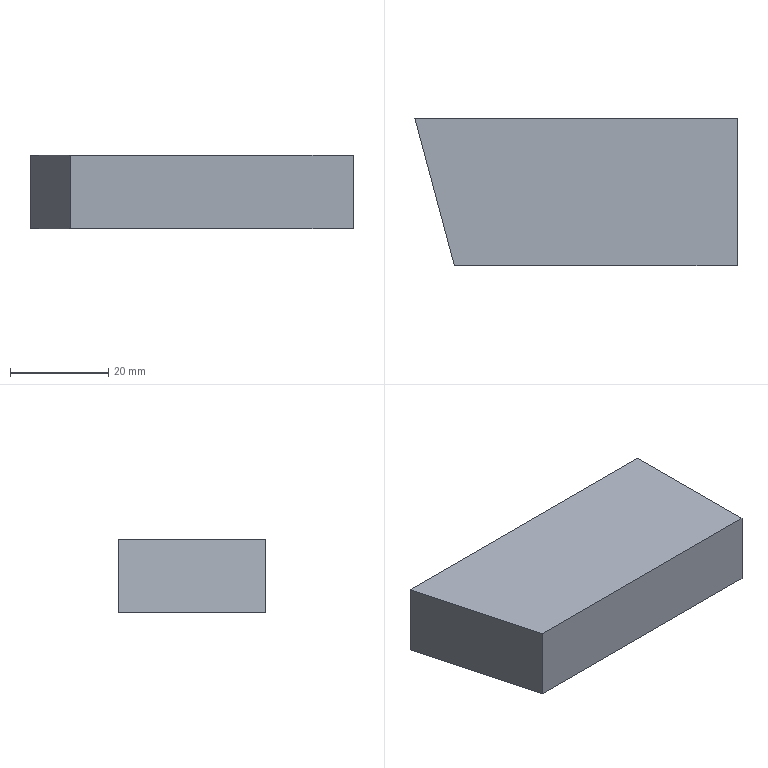Part | NX | features solid 2 | 1 solid | 6 faces | box 65.622 x 30 x 15 mm | volume 27721 mm3 | plane 6
STEP:
#1=CARTESIAN_POINT('',(-438.122,300.,-100.));
#2=VERTEX_POINT('',#1);
#3=CARTESIAN_POINT('',(-430.083,270.,-100.));
#4=VERTEX_POINT('',#3);
#5=CARTESIAN_POINT('',(-443.481,320.,-100.));
#6=DIRECTION('',(-0.2588,0.9659,0.));
#7=VECTOR('',#6,1000.);
#8=LINE('',#5,#7);
#9=EDGE_CURVE('',#2,#4,#8,.F.);
#10=ORIENTED_EDGE('',*,*,#9,.T.);
#11=CARTESIAN_POINT('',(-430.083,270.,-85.));
#12=VERTEX_POINT('',#11);
#13=CARTESIAN_POINT('',(-430.083,270.,-115.));
#14=DIRECTION('',(0.,0.,-1.));
#15=VECTOR('',#14,1000.);
#16=LINE('',#13,#15);
#17=EDGE_CURVE('',#4,#12,#16,.F.);
#18=ORIENTED_EDGE('',*,*,#17,.T.);
#19=CARTESIAN_POINT('',(-438.122,300.,-85.));
#20=VERTEX_POINT('',#19);
#21=CARTESIAN_POINT('',(-438.415,301.095,-85.));
#22=DIRECTION('',(0.2588,-0.9659,0.));
#23=VECTOR('',#22,1000.);
#24=LINE('',#21,#23);
#25=EDGE_CURVE('',#20,#12,#24,.T.);
#26=ORIENTED_EDGE('',*,*,#25,.F.);
#27=CARTESIAN_POINT('',(-438.122,300.,-115.));
#28=DIRECTION('',(0.,0.,-1.));
#29=VECTOR('',#28,1000.);
#30=LINE('',#27,#29);
#31=EDGE_CURVE('',#2,#20,#30,.F.);
#32=ORIENTED_EDGE('',*,*,#31,.F.);
#33=EDGE_LOOP('',(#10,#18,#26,#32));
#34=FACE_BOUND('',#33,.T.);
#35=CARTESIAN_POINT('',(-443.481,320.,-115.));
#36=DIRECTION('',(-0.9659,-0.2588,0.));
#37=DIRECTION('',(0.,0.,1.));
#38=AXIS2_PLACEMENT_3D('',#35,#36,#37);
#39=PLANE('',#38);
#40=ADVANCED_FACE('',(#34),#39,.T.);
#41=ORIENTED_EDGE('',*,*,#25,.T.);
#42=CARTESIAN_POINT('',(-372.5,270.,-85.));
#43=VERTEX_POINT('',#42);
#44=CARTESIAN_POINT('',(-442.5,270.,-85.));
#45=DIRECTION('',(-1.,0.,0.));
#46=VECTOR('',#45,1000.);
#47=LINE('',#44,#46);
#48=EDGE_CURVE('',#12,#43,#47,.F.);
#49=ORIENTED_EDGE('',*,*,#48,.T.);
#50=CARTESIAN_POINT('',(-372.5,300.,-85.));
#51=VERTEX_POINT('',#50);
#52=CARTESIAN_POINT('',(-372.5,50.,-85.));
#53=DIRECTION('',(0.,1.,0.));
#54=VECTOR('',#53,1000.);
#55=LINE('',#52,#54);
#56=EDGE_CURVE('',#51,#43,#55,.F.);
#57=ORIENTED_EDGE('',*,*,#56,.F.);
#58=CARTESIAN_POINT('',(-442.5,300.,-85.));
#59=DIRECTION('',(1.,0.,0.));
#60=VECTOR('',#59,1000.);
#61=LINE('',#58,#60);
#62=EDGE_CURVE('',#20,#51,#61,.T.);
#63=ORIENTED_EDGE('',*,*,#62,.F.);
#64=EDGE_LOOP('',(#41,#49,#57,#63));
#65=FACE_BOUND('',#64,.T.);
#66=CARTESIAN_POINT('',(-442.5,300.,-85.));
#67=DIRECTION('',(0.,0.,1.));
#68=DIRECTION('',(1.,0.,0.));
#69=AXIS2_PLACEMENT_3D('',#66,#67,#68);
#70=PLANE('',#69);
#71=ADVANCED_FACE('',(#65),#70,.T.);
#72=ORIENTED_EDGE('',*,*,#56,.T.);
#73=CARTESIAN_POINT('',(-372.5,270.,-100.));
#74=VERTEX_POINT('',#73);
#75=CARTESIAN_POINT('',(-372.5,270.,-100.));
#76=DIRECTION('',(0.,0.,1.));
#77=VECTOR('',#76,1000.);
#78=LINE('',#75,#77);
#79=EDGE_CURVE('',#74,#43,#78,.T.);
#80=ORIENTED_EDGE('',*,*,#79,.F.);
#81=CARTESIAN_POINT('',(-372.5,300.,-100.));
#82=VERTEX_POINT('',#81);
#83=CARTESIAN_POINT('',(-372.5,300.,-100.));
#84=DIRECTION('',(0.,-1.,0.));
#85=VECTOR('',#84,1000.);
#86=LINE('',#83,#85);
#87=EDGE_CURVE('',#82,#74,#86,.T.);
#88=ORIENTED_EDGE('',*,*,#87,.F.);
#89=CARTESIAN_POINT('',(-372.5,300.,-100.));
#90=DIRECTION('',(0.,0.,1.));
#91=VECTOR('',#90,1000.);
#92=LINE('',#89,#91);
#93=EDGE_CURVE('',#82,#51,#92,.T.);
#94=ORIENTED_EDGE('',*,*,#93,.T.);
#95=EDGE_LOOP('',(#72,#80,#88,#94));
#96=FACE_BOUND('',#95,.T.);
#97=CARTESIAN_POINT('',(-372.5,50.,-85.));
#98=DIRECTION('',(-1.,0.,0.));
#99=DIRECTION('',(0.,0.,1.));
#100=AXIS2_PLACEMENT_3D('',#97,#98,#99);
#101=PLANE('',#100);
#102=ADVANCED_FACE('',(#96),#101,.F.);
#103=CARTESIAN_POINT('',(-442.5,300.,-100.));
#104=DIRECTION('',(1.,0.,0.));
#105=VECTOR('',#104,1000.);
#106=LINE('',#103,#105);
#107=EDGE_CURVE('',#2,#82,#106,.T.);
#108=ORIENTED_EDGE('',*,*,#107,.T.);
#109=ORIENTED_EDGE('',*,*,#87,.T.);
#110=CARTESIAN_POINT('',(-442.5,270.,-100.));
#111=DIRECTION('',(1.,0.,0.));
#112=VECTOR('',#111,1000.);
#113=LINE('',#110,#112);
#114=EDGE_CURVE('',#4,#74,#113,.T.);
#115=ORIENTED_EDGE('',*,*,#114,.F.);
#116=ORIENTED_EDGE('',*,*,#9,.F.);
#117=EDGE_LOOP('',(#108,#109,#115,#116));
#118=FACE_BOUND('',#117,.T.);
#119=CARTESIAN_POINT('',(-442.5,300.,-100.));
#120=DIRECTION('',(0.,0.,1.));
#121=DIRECTION('',(1.,0.,0.));
#122=AXIS2_PLACEMENT_3D('',#119,#120,#121);
#123=PLANE('',#122);
#124=ADVANCED_FACE('',(#118),#123,.F.);
#125=ORIENTED_EDGE('',*,*,#79,.T.);
#126=ORIENTED_EDGE('',*,*,#48,.F.);
#127=ORIENTED_EDGE('',*,*,#17,.F.);
#128=ORIENTED_EDGE('',*,*,#114,.T.);
#129=EDGE_LOOP('',(#125,#126,#127,#128));
#130=FACE_BOUND('',#129,.T.);
#131=CARTESIAN_POINT('',(-442.5,270.,-100.));
#132=DIRECTION('',(0.,1.,0.));
#133=DIRECTION('',(0.,0.,1.));
#134=AXIS2_PLACEMENT_3D('',#131,#132,#133);
#135=PLANE('',#134);
#136=ADVANCED_FACE('',(#130),#135,.F.);
#137=ORIENTED_EDGE('',*,*,#93,.F.);
#138=ORIENTED_EDGE('',*,*,#107,.F.);
#139=ORIENTED_EDGE('',*,*,#31,.T.);
#140=ORIENTED_EDGE('',*,*,#62,.T.);
#141=EDGE_LOOP('',(#137,#138,#139,#140));
#142=FACE_BOUND('',#141,.T.);
#143=CARTESIAN_POINT('',(-442.5,300.,-100.));
#144=DIRECTION('',(0.,1.,0.));
#145=DIRECTION('',(0.,0.,1.));
#146=AXIS2_PLACEMENT_3D('',#143,#144,#145);
#147=PLANE('',#146);
#148=ADVANCED_FACE('',(#142),#147,.T.);
#149=CLOSED_SHELL('',(#40,#71,#102,#124,#136,#148));
#150=MANIFOLD_SOLID_BREP('',#149);
#151=(LENGTH_UNIT()NAMED_UNIT(*)SI_UNIT(.MILLI.,.METRE.));
#152=UNCERTAINTY_MEASURE_WITH_UNIT(LENGTH_MEASURE(0.00001),#151,'','');
#153=(NAMED_UNIT(*)PLANE_ANGLE_UNIT()SI_UNIT($,.RADIAN.));
#154=(NAMED_UNIT(*)SI_UNIT($,.STERADIAN.)SOLID_ANGLE_UNIT());
#155=(GEOMETRIC_REPRESENTATION_CONTEXT(3)GLOBAL_UNCERTAINTY_ASSIGNED_CONTEXT((#152))GLOBAL_UNIT_ASSIGNED_CONTEXT((#151,#153,#154))REPRESENTATION_CONTEXT('',''));
#156=ADVANCED_BREP_SHAPE_REPRESENTATION('',(#150),#155);